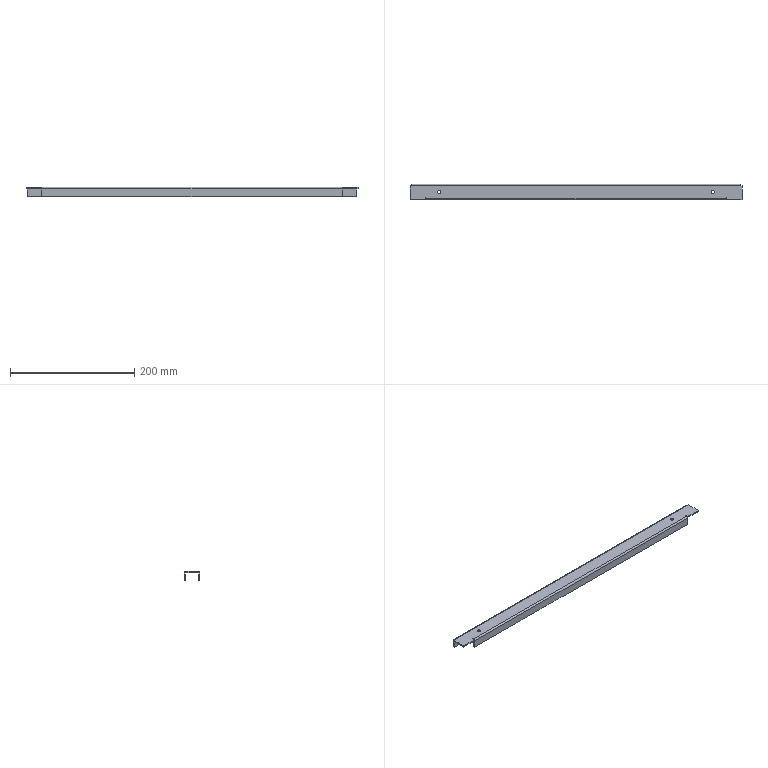Part | STEP file | Clamp Frame Weldment 1 | 1 solid | 30 faces | box 534 x 25 x 15 mm | volume 51628 mm3 | plane 20 | cylinder 10 | commonest cylinder face diameters 1 x4 5.2 x4 5 x2
STEP:
#1=CARTESIAN_POINT('',(-67.6,850.6,-2.));
#2=VERTEX_POINT('',#1);
#3=CARTESIAN_POINT('',(-62.4,850.6,-2.));
#4=VERTEX_POINT('',#3);
#5=CARTESIAN_POINT('',(-65.,850.6,-2.));
#6=DIRECTION('',(0.,0.,1.));
#7=DIRECTION('',(1.,0.,0.));
#8=AXIS2_PLACEMENT_3D('',#5,#6,#7);
#9=CIRCLE('',#8,2.6);
#10=EDGE_CURVE('',#2,#4,#9,.T.);
#11=ORIENTED_EDGE('',*,*,#10,.F.);
#12=CARTESIAN_POINT('',(-67.6,850.6,0.));
#13=VERTEX_POINT('',#12);
#14=CARTESIAN_POINT('',(-67.6,850.6,-10.));
#15=DIRECTION('',(0.,0.,1.));
#16=VECTOR('',#15,1000.);
#17=LINE('',#14,#16);
#18=EDGE_CURVE('',#2,#13,#17,.T.);
#19=ORIENTED_EDGE('',*,*,#18,.T.);
#20=CARTESIAN_POINT('',(-62.4,850.6,0.));
#21=VERTEX_POINT('',#20);
#22=CARTESIAN_POINT('',(-65.,850.6,0.));
#23=DIRECTION('',(0.,0.,1.));
#24=DIRECTION('',(1.,0.,0.));
#25=AXIS2_PLACEMENT_3D('',#22,#23,#24);
#26=CIRCLE('',#25,2.6);
#27=EDGE_CURVE('',#13,#21,#26,.T.);
#28=ORIENTED_EDGE('',*,*,#27,.T.);
#29=CARTESIAN_POINT('',(-62.4,850.6,-10.));
#30=DIRECTION('',(0.,0.,1.));
#31=VECTOR('',#30,1000.);
#32=LINE('',#29,#31);
#33=EDGE_CURVE('',#4,#21,#32,.T.);
#34=ORIENTED_EDGE('',*,*,#33,.F.);
#35=EDGE_LOOP('',(#11,#19,#28,#34));
#36=FACE_OUTER_BOUND('',#35,.T.);
#37=CARTESIAN_POINT('',(-65.,850.6,-10.));
#38=DIRECTION('',(0.,0.,1.));
#39=DIRECTION('',(1.,0.,0.));
#40=AXIS2_PLACEMENT_3D('',#37,#38,#39);
#41=CYLINDRICAL_SURFACE('',#40,2.6);
#42=ADVANCED_FACE('',(#36),#41,.F.);
#43=CARTESIAN_POINT('',(-507.6,850.6,-2.));
#44=VERTEX_POINT('',#43);
#45=CARTESIAN_POINT('',(-502.4,850.6,-2.));
#46=VERTEX_POINT('',#45);
#47=CARTESIAN_POINT('',(-505.,850.6,-2.));
#48=DIRECTION('',(0.,0.,1.));
#49=DIRECTION('',(1.,0.,0.));
#50=AXIS2_PLACEMENT_3D('',#47,#48,#49);
#51=CIRCLE('',#50,2.6);
#52=EDGE_CURVE('',#44,#46,#51,.T.);
#53=ORIENTED_EDGE('',*,*,#52,.F.);
#54=CARTESIAN_POINT('',(-507.6,850.6,0.));
#55=VERTEX_POINT('',#54);
#56=CARTESIAN_POINT('',(-507.6,850.6,-10.));
#57=DIRECTION('',(0.,0.,1.));
#58=VECTOR('',#57,1000.);
#59=LINE('',#56,#58);
#60=EDGE_CURVE('',#44,#55,#59,.T.);
#61=ORIENTED_EDGE('',*,*,#60,.T.);
#62=CARTESIAN_POINT('',(-502.4,850.6,0.));
#63=VERTEX_POINT('',#62);
#64=CARTESIAN_POINT('',(-505.,850.6,0.));
#65=DIRECTION('',(0.,0.,1.));
#66=DIRECTION('',(1.,0.,0.));
#67=AXIS2_PLACEMENT_3D('',#64,#65,#66);
#68=CIRCLE('',#67,2.6);
#69=EDGE_CURVE('',#55,#63,#68,.T.);
#70=ORIENTED_EDGE('',*,*,#69,.T.);
#71=CARTESIAN_POINT('',(-502.4,850.6,-10.));
#72=DIRECTION('',(0.,0.,1.));
#73=VECTOR('',#72,1000.);
#74=LINE('',#71,#73);
#75=EDGE_CURVE('',#46,#63,#74,.T.);
#76=ORIENTED_EDGE('',*,*,#75,.F.);
#77=EDGE_LOOP('',(#53,#61,#70,#76));
#78=FACE_OUTER_BOUND('',#77,.T.);
#79=CARTESIAN_POINT('',(-505.,850.6,-10.));
#80=DIRECTION('',(0.,0.,1.));
#81=DIRECTION('',(1.,0.,0.));
#82=AXIS2_PLACEMENT_3D('',#79,#80,#81);
#83=CYLINDRICAL_SURFACE('',#82,2.6);
#84=ADVANCED_FACE('',(#78),#83,.F.);
#85=CARTESIAN_POINT('',(-527.8,841.6,0.));
#86=VERTEX_POINT('',#85);
#87=CARTESIAN_POINT('',(-526.8,841.6,0.));
#88=VERTEX_POINT('',#87);
#89=CARTESIAN_POINT('',(-527.3,841.6,0.));
#90=DIRECTION('',(0.,0.,-1.));
#91=DIRECTION('',(1.,0.,0.));
#92=AXIS2_PLACEMENT_3D('',#89,#90,#91);
#93=CIRCLE('',#92,0.5);
#94=EDGE_CURVE('',#86,#88,#93,.T.);
#95=ORIENTED_EDGE('',*,*,#94,.T.);
#96=CARTESIAN_POINT('',(-526.8,840.6,0.));
#97=VERTEX_POINT('',#96);
#98=CARTESIAN_POINT('',(-526.8,841.6,0.));
#99=DIRECTION('',(0.,1.,0.));
#100=VECTOR('',#99,1000.);
#101=LINE('',#98,#100);
#102=EDGE_CURVE('',#97,#88,#101,.T.);
#103=ORIENTED_EDGE('',*,*,#102,.F.);
#104=CARTESIAN_POINT('',(-43.2,840.6,0.));
#105=VERTEX_POINT('',#104);
#106=CARTESIAN_POINT('',(0.,840.6,0.));
#107=DIRECTION('',(-1.,0.,0.));
#108=VECTOR('',#107,1000.);
#109=LINE('',#106,#108);
#110=EDGE_CURVE('',#105,#97,#109,.T.);
#111=ORIENTED_EDGE('',*,*,#110,.F.);
#112=CARTESIAN_POINT('',(-43.2,841.6,0.));
#113=VERTEX_POINT('',#112);
#114=CARTESIAN_POINT('',(-43.2,840.6,0.));
#115=DIRECTION('',(0.,-1.,0.));
#116=VECTOR('',#115,1000.);
#117=LINE('',#114,#116);
#118=EDGE_CURVE('',#113,#105,#117,.T.);
#119=ORIENTED_EDGE('',*,*,#118,.F.);
#120=CARTESIAN_POINT('',(-42.2,841.6,0.));
#121=VERTEX_POINT('',#120);
#122=CARTESIAN_POINT('',(-42.7,841.6,0.));
#123=DIRECTION('',(0.,0.,-1.));
#124=DIRECTION('',(1.,0.,0.));
#125=AXIS2_PLACEMENT_3D('',#122,#123,#124);
#126=CIRCLE('',#125,0.5);
#127=EDGE_CURVE('',#113,#121,#126,.T.);
#128=ORIENTED_EDGE('',*,*,#127,.T.);
#129=CARTESIAN_POINT('',(-42.2,838.1,0.));
#130=VERTEX_POINT('',#129);
#131=CARTESIAN_POINT('',(-42.2,0.,0.));
#132=DIRECTION('',(0.,1.,0.));
#133=VECTOR('',#132,1000.);
#134=LINE('',#131,#133);
#135=EDGE_CURVE('',#130,#121,#134,.T.);
#136=ORIENTED_EDGE('',*,*,#135,.F.);
#137=CARTESIAN_POINT('',(-18.,838.1,0.));
#138=VERTEX_POINT('',#137);
#139=CARTESIAN_POINT('',(0.,838.1,0.));
#140=DIRECTION('',(-1.,0.,0.));
#141=VECTOR('',#140,1000.);
#142=LINE('',#139,#141);
#143=EDGE_CURVE('',#138,#130,#142,.T.);
#144=ORIENTED_EDGE('',*,*,#143,.F.);
#145=CARTESIAN_POINT('',(-18.,860.6,0.));
#146=VERTEX_POINT('',#145);
#147=CARTESIAN_POINT('',(-18.,0.,0.));
#148=DIRECTION('',(0.,-1.,0.));
#149=VECTOR('',#148,1000.);
#150=LINE('',#147,#149);
#151=EDGE_CURVE('',#146,#138,#150,.T.);
#152=ORIENTED_EDGE('',*,*,#151,.F.);
#153=CARTESIAN_POINT('',(-20.,860.6,0.));
#154=VERTEX_POINT('',#153);
#155=CARTESIAN_POINT('',(0.,860.6,0.));
#156=DIRECTION('',(1.,0.,0.));
#157=VECTOR('',#156,1000.);
#158=LINE('',#155,#157);
#159=EDGE_CURVE('',#154,#146,#158,.T.);
#160=ORIENTED_EDGE('',*,*,#159,.F.);
#161=CARTESIAN_POINT('',(-550.,860.6,0.));
#162=VERTEX_POINT('',#161);
#163=CARTESIAN_POINT('',(0.,860.6,0.));
#164=DIRECTION('',(1.,0.,0.));
#165=VECTOR('',#164,1000.);
#166=LINE('',#163,#165);
#167=EDGE_CURVE('',#162,#154,#166,.T.);
#168=ORIENTED_EDGE('',*,*,#167,.F.);
#169=CARTESIAN_POINT('',(-552.,860.6,0.));
#170=VERTEX_POINT('',#169);
#171=CARTESIAN_POINT('',(0.,860.6,0.));
#172=DIRECTION('',(1.,0.,0.));
#173=VECTOR('',#172,1000.);
#174=LINE('',#171,#173);
#175=EDGE_CURVE('',#170,#162,#174,.T.);
#176=ORIENTED_EDGE('',*,*,#175,.F.);
#177=CARTESIAN_POINT('',(-552.,838.1,0.));
#178=VERTEX_POINT('',#177);
#179=CARTESIAN_POINT('',(-552.,0.,0.));
#180=DIRECTION('',(0.,1.,0.));
#181=VECTOR('',#180,1000.);
#182=LINE('',#179,#181);
#183=EDGE_CURVE('',#178,#170,#182,.T.);
#184=ORIENTED_EDGE('',*,*,#183,.F.);
#185=CARTESIAN_POINT('',(-527.8,838.1,0.));
#186=VERTEX_POINT('',#185);
#187=CARTESIAN_POINT('',(0.,838.1,0.));
#188=DIRECTION('',(-1.,0.,0.));
#189=VECTOR('',#188,1000.);
#190=LINE('',#187,#189);
#191=EDGE_CURVE('',#186,#178,#190,.T.);
#192=ORIENTED_EDGE('',*,*,#191,.F.);
#193=CARTESIAN_POINT('',(-527.8,0.,0.));
#194=DIRECTION('',(0.,-1.,0.));
#195=VECTOR('',#194,1000.);
#196=LINE('',#193,#195);
#197=EDGE_CURVE('',#86,#186,#196,.T.);
#198=ORIENTED_EDGE('',*,*,#197,.F.);
#199=EDGE_LOOP('',(#95,#103,#111,#119,#128,#136,#144,#152,#160,#168,#176,#184,#192,#198));
#200=FACE_OUTER_BOUND('',#199,.T.);
#201=CARTESIAN_POINT('',(-65.,850.6,0.));
#202=DIRECTION('',(0.,0.,1.));
#203=DIRECTION('',(1.,0.,0.));
#204=AXIS2_PLACEMENT_3D('',#201,#202,#203);
#205=CIRCLE('',#204,2.6);
#206=EDGE_CURVE('',#21,#13,#205,.T.);
#207=ORIENTED_EDGE('',*,*,#206,.F.);
#208=ORIENTED_EDGE('',*,*,#27,.F.);
#209=EDGE_LOOP('',(#207,#208));
#210=FACE_BOUND('',#209,.T.);
#211=CARTESIAN_POINT('',(-505.,850.6,0.));
#212=DIRECTION('',(0.,0.,1.));
#213=DIRECTION('',(1.,0.,0.));
#214=AXIS2_PLACEMENT_3D('',#211,#212,#213);
#215=CIRCLE('',#214,2.6);
#216=EDGE_CURVE('',#63,#55,#215,.T.);
#217=ORIENTED_EDGE('',*,*,#216,.F.);
#218=ORIENTED_EDGE('',*,*,#69,.F.);
#219=EDGE_LOOP('',(#217,#218));
#220=FACE_BOUND('',#219,.T.);
#221=CARTESIAN_POINT('',(0.,0.,0.));
#222=DIRECTION('',(0.,0.,-1.));
#223=DIRECTION('',(-1.,0.,0.));
#224=AXIS2_PLACEMENT_3D('',#221,#222,#223);
#225=PLANE('',#224);
#226=ADVANCED_FACE('',(#200,#210,#220),#225,.F.);
#227=CARTESIAN_POINT('',(-527.8,838.1,-2.));
#228=VERTEX_POINT('',#227);
#229=CARTESIAN_POINT('',(-527.8,838.1,-2.));
#230=DIRECTION('',(0.,0.,-1.));
#231=VECTOR('',#230,1000.);
#232=LINE('',#229,#231);
#233=EDGE_CURVE('',#186,#228,#232,.T.);
#234=ORIENTED_EDGE('',*,*,#233,.T.);
#235=CARTESIAN_POINT('',(-527.8,841.6,-2.));
#236=VERTEX_POINT('',#235);
#237=CARTESIAN_POINT('',(-527.8,838.1,-2.));
#238=DIRECTION('',(0.,1.,0.));
#239=VECTOR('',#238,1000.);
#240=LINE('',#237,#239);
#241=EDGE_CURVE('',#228,#236,#240,.T.);
#242=ORIENTED_EDGE('',*,*,#241,.T.);
#243=CARTESIAN_POINT('',(-527.8,841.6,-2.));
#244=DIRECTION('',(0.,0.,1.));
#245=VECTOR('',#244,1000.);
#246=LINE('',#243,#245);
#247=EDGE_CURVE('',#236,#86,#246,.T.);
#248=ORIENTED_EDGE('',*,*,#247,.T.);
#249=ORIENTED_EDGE('',*,*,#197,.T.);
#250=EDGE_LOOP('',(#234,#242,#248,#249));
#251=FACE_OUTER_BOUND('',#250,.T.);
#252=CARTESIAN_POINT('',(-527.8,838.1,-2.));
#253=DIRECTION('',(1.,0.,0.));
#254=DIRECTION('',(0.,0.,-1.));
#255=AXIS2_PLACEMENT_3D('',#252,#253,#254);
#256=PLANE('',#255);
#257=ADVANCED_FACE('',(#251),#256,.T.);
#258=CARTESIAN_POINT('',(-526.8,838.1,-2.5));
#259=VERTEX_POINT('',#258);
#260=CARTESIAN_POINT('',(-43.2,838.1,-2.5));
#261=VERTEX_POINT('',#260);
#262=CARTESIAN_POINT('',(-526.8,838.1,-2.5));
#263=DIRECTION('',(1.,0.,0.));
#264=VECTOR('',#263,1000.);
#265=LINE('',#262,#264);
#266=EDGE_CURVE('',#259,#261,#265,.T.);
#267=ORIENTED_EDGE('',*,*,#266,.T.);
#268=CARTESIAN_POINT('',(-43.2,840.6,-2.5));
#269=DIRECTION('',(-1.,0.,0.));
#270=DIRECTION('',(0.,0.,1.));
#271=AXIS2_PLACEMENT_3D('',#268,#269,#270);
#272=CIRCLE('',#271,2.5);
#273=EDGE_CURVE('',#261,#105,#272,.T.);
#274=ORIENTED_EDGE('',*,*,#273,.T.);
#275=ORIENTED_EDGE('',*,*,#110,.T.);
#276=CARTESIAN_POINT('',(-526.8,840.6,-2.5));
#277=DIRECTION('',(1.,0.,0.));
#278=DIRECTION('',(0.,0.,1.));
#279=AXIS2_PLACEMENT_3D('',#276,#277,#278);
#280=CIRCLE('',#279,2.5);
#281=EDGE_CURVE('',#97,#259,#280,.T.);
#282=ORIENTED_EDGE('',*,*,#281,.T.);
#283=EDGE_LOOP('',(#267,#274,#275,#282));
#284=FACE_OUTER_BOUND('',#283,.T.);
#285=CARTESIAN_POINT('',(-526.8,840.6,-2.5));
#286=DIRECTION('',(-1.,0.,0.));
#287=DIRECTION('',(0.,0.,1.));
#288=AXIS2_PLACEMENT_3D('',#285,#286,#287);
#289=CYLINDRICAL_SURFACE('',#288,2.5);
#290=ADVANCED_FACE('',(#284),#289,.T.);
#291=CARTESIAN_POINT('',(-42.2,841.6,-2.));
#292=VERTEX_POINT('',#291);
#293=CARTESIAN_POINT('',(-42.2,841.6,-2.));
#294=DIRECTION('',(0.,0.,-1.));
#295=VECTOR('',#294,1000.);
#296=LINE('',#293,#295);
#297=EDGE_CURVE('',#121,#292,#296,.T.);
#298=ORIENTED_EDGE('',*,*,#297,.T.);
#299=CARTESIAN_POINT('',(-42.2,838.1,-2.));
#300=VERTEX_POINT('',#299);
#301=CARTESIAN_POINT('',(-42.2,841.6,-2.));
#302=DIRECTION('',(0.,-1.,0.));
#303=VECTOR('',#302,1000.);
#304=LINE('',#301,#303);
#305=EDGE_CURVE('',#292,#300,#304,.T.);
#306=ORIENTED_EDGE('',*,*,#305,.T.);
#307=CARTESIAN_POINT('',(-42.2,838.1,-2.));
#308=DIRECTION('',(0.,0.,1.));
#309=VECTOR('',#308,1000.);
#310=LINE('',#307,#309);
#311=EDGE_CURVE('',#300,#130,#310,.T.);
#312=ORIENTED_EDGE('',*,*,#311,.T.);
#313=ORIENTED_EDGE('',*,*,#135,.T.);
#314=EDGE_LOOP('',(#298,#306,#312,#313));
#315=FACE_OUTER_BOUND('',#314,.T.);
#316=CARTESIAN_POINT('',(-42.2,841.6,-2.));
#317=DIRECTION('',(-1.,0.,0.));
#318=DIRECTION('',(0.,0.,1.));
#319=AXIS2_PLACEMENT_3D('',#316,#317,#318);
#320=PLANE('',#319);
#321=ADVANCED_FACE('',(#315),#320,.T.);
#322=CARTESIAN_POINT('',(-18.,838.1,-2.));
#323=VERTEX_POINT('',#322);
#324=CARTESIAN_POINT('',(-18.,838.1,-2.));
#325=DIRECTION('',(0.,0.,1.));
#326=VECTOR('',#325,1000.);
#327=LINE('',#324,#326);
#328=EDGE_CURVE('',#323,#138,#327,.T.);
#329=ORIENTED_EDGE('',*,*,#328,.T.);
#330=ORIENTED_EDGE('',*,*,#143,.T.);
#331=ORIENTED_EDGE('',*,*,#311,.F.);
#332=CARTESIAN_POINT('',(-43.,838.1,-2.));
#333=DIRECTION('',(1.,0.,0.));
#334=VECTOR('',#333,1000.);
#335=LINE('',#332,#334);
#336=EDGE_CURVE('',#300,#323,#335,.T.);
#337=ORIENTED_EDGE('',*,*,#336,.T.);
#338=EDGE_LOOP('',(#329,#330,#331,#337));
#339=FACE_OUTER_BOUND('',#338,.T.);
#340=CARTESIAN_POINT('',(-43.,838.1,-2.));
#341=DIRECTION('',(0.,-1.,0.));
#342=DIRECTION('',(0.,0.,-1.));
#343=AXIS2_PLACEMENT_3D('',#340,#341,#342);
#344=PLANE('',#343);
#345=ADVANCED_FACE('',(#339),#344,.T.);
#346=CARTESIAN_POINT('',(-18.,860.6,-2.));
#347=VERTEX_POINT('',#346);
#348=CARTESIAN_POINT('',(-18.,860.6,0.));
#349=DIRECTION('',(0.,0.,1.));
#350=VECTOR('',#349,1000.);
#351=LINE('',#348,#350);
#352=EDGE_CURVE('',#347,#146,#351,.T.);
#353=ORIENTED_EDGE('',*,*,#352,.T.);
#354=ORIENTED_EDGE('',*,*,#151,.T.);
#355=ORIENTED_EDGE('',*,*,#328,.F.);
#356=CARTESIAN_POINT('',(-18.,0.,-2.));
#357=DIRECTION('',(0.,1.,0.));
#358=VECTOR('',#357,1000.);
#359=LINE('',#356,#358);
#360=EDGE_CURVE('',#323,#347,#359,.T.);
#361=ORIENTED_EDGE('',*,*,#360,.T.);
#362=EDGE_LOOP('',(#353,#354,#355,#361));
#363=FACE_OUTER_BOUND('',#362,.T.);
#364=CARTESIAN_POINT('',(-18.,0.,0.));
#365=DIRECTION('',(1.,0.,0.));
#366=DIRECTION('',(0.,1.,0.));
#367=AXIS2_PLACEMENT_3D('',#364,#365,#366);
#368=PLANE('',#367);
#369=ADVANCED_FACE('',(#363),#368,.T.);
#370=ORIENTED_EDGE('',*,*,#159,.T.);
#371=ORIENTED_EDGE('',*,*,#352,.F.);
#372=CARTESIAN_POINT('',(-20.,860.6,-2.));
#373=VERTEX_POINT('',#372);
#374=CARTESIAN_POINT('',(-18.,860.6,-2.));
#375=DIRECTION('',(1.,0.,0.));
#376=VECTOR('',#375,1000.);
#377=LINE('',#374,#376);
#378=EDGE_CURVE('',#373,#347,#377,.T.);
#379=ORIENTED_EDGE('',*,*,#378,.F.);
#380=CARTESIAN_POINT('',(-20.,860.6,-2.));
#381=DIRECTION('',(0.,0.,-1.));
#382=VECTOR('',#381,1000.);
#383=LINE('',#380,#382);
#384=EDGE_CURVE('',#154,#373,#383,.T.);
#385=ORIENTED_EDGE('',*,*,#384,.F.);
#386=EDGE_LOOP('',(#370,#371,#379,#385));
#387=FACE_OUTER_BOUND('',#386,.T.);
#388=CARTESIAN_POINT('',(-18.,860.6,-2.));
#389=DIRECTION('',(0.,-1.,0.));
#390=DIRECTION('',(1.,0.,0.));
#391=AXIS2_PLACEMENT_3D('',#388,#389,#390);
#392=PLANE('',#391);
#393=ADVANCED_FACE('',(#387),#392,.F.);
#394=CARTESIAN_POINT('',(-20.,863.1,-2.5));
#395=VERTEX_POINT('',#394);
#396=CARTESIAN_POINT('',(-550.,863.1,-2.5));
#397=VERTEX_POINT('',#396);
#398=CARTESIAN_POINT('',(-20.,863.1,-2.5));
#399=DIRECTION('',(-1.,0.,0.));
#400=VECTOR('',#399,1000.);
#401=LINE('',#398,#400);
#402=EDGE_CURVE('',#395,#397,#401,.T.);
#403=ORIENTED_EDGE('',*,*,#402,.T.);
#404=CARTESIAN_POINT('',(-550.,860.6,-2.5));
#405=DIRECTION('',(1.,0.,0.));
#406=DIRECTION('',(0.,0.,-1.));
#407=AXIS2_PLACEMENT_3D('',#404,#405,#406);
#408=CIRCLE('',#407,2.5);
#409=EDGE_CURVE('',#397,#162,#408,.T.);
#410=ORIENTED_EDGE('',*,*,#409,.T.);
#411=ORIENTED_EDGE('',*,*,#167,.T.);
#412=CARTESIAN_POINT('',(-20.,860.6,-2.5));
#413=DIRECTION('',(-1.,0.,0.));
#414=DIRECTION('',(0.,0.,-1.));
#415=AXIS2_PLACEMENT_3D('',#412,#413,#414);
#416=CIRCLE('',#415,2.5);
#417=EDGE_CURVE('',#154,#395,#416,.T.);
#418=ORIENTED_EDGE('',*,*,#417,.T.);
#419=EDGE_LOOP('',(#403,#410,#411,#418));
#420=FACE_OUTER_BOUND('',#419,.T.);
#421=CARTESIAN_POINT('',(-20.,860.6,-2.5));
#422=DIRECTION('',(1.,0.,0.));
#423=DIRECTION('',(0.,0.,-1.));
#424=AXIS2_PLACEMENT_3D('',#421,#422,#423);
#425=CYLINDRICAL_SURFACE('',#424,2.5);
#426=ADVANCED_FACE('',(#420),#425,.T.);
#427=CARTESIAN_POINT('',(-552.,860.6,-2.));
#428=VERTEX_POINT('',#427);
#429=CARTESIAN_POINT('',(-550.,860.6,-2.));
#430=VERTEX_POINT('',#429);
#431=CARTESIAN_POINT('',(-552.,860.6,-2.));
#432=DIRECTION('',(1.,0.,0.));
#433=VECTOR('',#432,1000.);
#434=LINE('',#431,#433);
#435=EDGE_CURVE('',#428,#430,#434,.T.);
#436=ORIENTED_EDGE('',*,*,#435,.F.);
#437=CARTESIAN_POINT('',(-552.,860.6,0.));
#438=DIRECTION('',(0.,0.,-1.));
#439=VECTOR('',#438,1000.);
#440=LINE('',#437,#439);
#441=EDGE_CURVE('',#170,#428,#440,.T.);
#442=ORIENTED_EDGE('',*,*,#441,.F.);
#443=ORIENTED_EDGE('',*,*,#175,.T.);
#444=CARTESIAN_POINT('',(-550.,860.6,0.));
#445=DIRECTION('',(0.,0.,1.));
#446=VECTOR('',#445,1000.);
#447=LINE('',#444,#446);
#448=EDGE_CURVE('',#430,#162,#447,.T.);
#449=ORIENTED_EDGE('',*,*,#448,.F.);
#450=EDGE_LOOP('',(#436,#442,#443,#449));
#451=FACE_OUTER_BOUND('',#450,.T.);
#452=CARTESIAN_POINT('',(-552.,860.6,0.));
#453=DIRECTION('',(0.,-1.,0.));
#454=DIRECTION('',(0.,0.,-1.));
#455=AXIS2_PLACEMENT_3D('',#452,#453,#454);
#456=PLANE('',#455);
#457=ADVANCED_FACE('',(#451),#456,.F.);
#458=CARTESIAN_POINT('',(-552.,838.1,-2.));
#459=VERTEX_POINT('',#458);
#460=CARTESIAN_POINT('',(-552.,0.,-2.));
#461=DIRECTION('',(0.,-1.,0.));
#462=VECTOR('',#461,1000.);
#463=LINE('',#460,#462);
#464=EDGE_CURVE('',#428,#459,#463,.T.);
#465=ORIENTED_EDGE('',*,*,#464,.T.);
#466=CARTESIAN_POINT('',(-552.,838.1,0.));
#467=DIRECTION('',(0.,0.,1.));
#468=VECTOR('',#467,1000.);
#469=LINE('',#466,#468);
#470=EDGE_CURVE('',#459,#178,#469,.T.);
#471=ORIENTED_EDGE('',*,*,#470,.T.);
#472=ORIENTED_EDGE('',*,*,#183,.T.);
#473=ORIENTED_EDGE('',*,*,#441,.T.);
#474=EDGE_LOOP('',(#465,#471,#472,#473));
#475=FACE_OUTER_BOUND('',#474,.T.);
#476=CARTESIAN_POINT('',(-552.,0.,0.));
#477=DIRECTION('',(-1.,0.,0.));
#478=DIRECTION('',(0.,0.,1.));
#479=AXIS2_PLACEMENT_3D('',#476,#477,#478);
#480=PLANE('',#479);
#481=ADVANCED_FACE('',(#475),#480,.T.);
#482=ORIENTED_EDGE('',*,*,#191,.T.);
#483=ORIENTED_EDGE('',*,*,#470,.F.);
#484=CARTESIAN_POINT('',(-550.,838.1,-2.));
#485=DIRECTION('',(1.,0.,0.));
#486=VECTOR('',#485,1000.);
#487=LINE('',#484,#486);
#488=EDGE_CURVE('',#459,#228,#487,.T.);
#489=ORIENTED_EDGE('',*,*,#488,.T.);
#490=ORIENTED_EDGE('',*,*,#233,.F.);
#491=EDGE_LOOP('',(#482,#483,#489,#490));
#492=FACE_OUTER_BOUND('',#491,.T.);
#493=CARTESIAN_POINT('',(-550.,838.1,-2.));
#494=DIRECTION('',(0.,-1.,0.));
#495=DIRECTION('',(1.,0.,0.));
#496=AXIS2_PLACEMENT_3D('',#493,#494,#495);
#497=PLANE('',#496);
#498=ADVANCED_FACE('',(#492),#497,.T.);
#499=ORIENTED_EDGE('',*,*,#18,.F.);
#500=CARTESIAN_POINT('',(-65.,850.6,-2.));
#501=DIRECTION('',(0.,0.,1.));
#502=DIRECTION('',(1.,0.,0.));
#503=AXIS2_PLACEMENT_3D('',#500,#501,#502);
#504=CIRCLE('',#503,2.6);
#505=EDGE_CURVE('',#4,#2,#504,.T.);
#506=ORIENTED_EDGE('',*,*,#505,.F.);
#507=ORIENTED_EDGE('',*,*,#33,.T.);
#508=ORIENTED_EDGE('',*,*,#206,.T.);
#509=EDGE_LOOP('',(#499,#506,#507,#508));
#510=FACE_OUTER_BOUND('',#509,.T.);
#511=CARTESIAN_POINT('',(-65.,850.6,-10.));
#512=DIRECTION('',(0.,0.,1.));
#513=DIRECTION('',(1.,0.,0.));
#514=AXIS2_PLACEMENT_3D('',#511,#512,#513);
#515=CYLINDRICAL_SURFACE('',#514,2.6);
#516=ADVANCED_FACE('',(#510),#515,.F.);
#517=ORIENTED_EDGE('',*,*,#60,.F.);
#518=CARTESIAN_POINT('',(-505.,850.6,-2.));
#519=DIRECTION('',(0.,0.,1.));
#520=DIRECTION('',(1.,0.,0.));
#521=AXIS2_PLACEMENT_3D('',#518,#519,#520);
#522=CIRCLE('',#521,2.6);
#523=EDGE_CURVE('',#46,#44,#522,.T.);
#524=ORIENTED_EDGE('',*,*,#523,.F.);
#525=ORIENTED_EDGE('',*,*,#75,.T.);
#526=ORIENTED_EDGE('',*,*,#216,.T.);
#527=EDGE_LOOP('',(#517,#524,#525,#526));
#528=FACE_OUTER_BOUND('',#527,.T.);
#529=CARTESIAN_POINT('',(-505.,850.6,-10.));
#530=DIRECTION('',(0.,0.,1.));
#531=DIRECTION('',(1.,0.,0.));
#532=AXIS2_PLACEMENT_3D('',#529,#530,#531);
#533=CYLINDRICAL_SURFACE('',#532,2.6);
#534=ADVANCED_FACE('',(#528),#533,.F.);
#535=CARTESIAN_POINT('',(-43.2,840.6,-2.));
#536=VERTEX_POINT('',#535);
#537=CARTESIAN_POINT('',(-526.8,840.6,-2.));
#538=VERTEX_POINT('',#537);
#539=CARTESIAN_POINT('',(0.,840.6,-2.));
#540=DIRECTION('',(-1.,0.,0.));
#541=VECTOR('',#540,1000.);
#542=LINE('',#539,#541);
#543=EDGE_CURVE('',#536,#538,#542,.T.);
#544=ORIENTED_EDGE('',*,*,#543,.T.);
#545=CARTESIAN_POINT('',(-526.8,841.6,-2.));
#546=VERTEX_POINT('',#545);
#547=CARTESIAN_POINT('',(-526.8,841.6,-2.));
#548=DIRECTION('',(0.,-1.,0.));
#549=VECTOR('',#548,1000.);
#550=LINE('',#547,#549);
#551=EDGE_CURVE('',#546,#538,#550,.T.);
#552=ORIENTED_EDGE('',*,*,#551,.F.);
#553=CARTESIAN_POINT('',(-527.3,841.6,-2.));
#554=DIRECTION('',(0.,0.,1.));
#555=DIRECTION('',(1.,0.,0.));
#556=AXIS2_PLACEMENT_3D('',#553,#554,#555);
#557=CIRCLE('',#556,0.5);
#558=EDGE_CURVE('',#546,#236,#557,.T.);
#559=ORIENTED_EDGE('',*,*,#558,.T.);
#560=ORIENTED_EDGE('',*,*,#241,.F.);
#561=ORIENTED_EDGE('',*,*,#488,.F.);
#562=ORIENTED_EDGE('',*,*,#464,.F.);
#563=ORIENTED_EDGE('',*,*,#435,.T.);
#564=CARTESIAN_POINT('',(0.,860.6,-2.));
#565=DIRECTION('',(1.,0.,0.));
#566=VECTOR('',#565,1000.);
#567=LINE('',#564,#566);
#568=EDGE_CURVE('',#430,#373,#567,.T.);
#569=ORIENTED_EDGE('',*,*,#568,.T.);
#570=ORIENTED_EDGE('',*,*,#378,.T.);
#571=ORIENTED_EDGE('',*,*,#360,.F.);
#572=ORIENTED_EDGE('',*,*,#336,.F.);
#573=ORIENTED_EDGE('',*,*,#305,.F.);
#574=CARTESIAN_POINT('',(-43.2,841.6,-2.));
#575=VERTEX_POINT('',#574);
#576=CARTESIAN_POINT('',(-42.7,841.6,-2.));
#577=DIRECTION('',(0.,0.,1.));
#578=DIRECTION('',(1.,0.,0.));
#579=AXIS2_PLACEMENT_3D('',#576,#577,#578);
#580=CIRCLE('',#579,0.5);
#581=EDGE_CURVE('',#292,#575,#580,.T.);
#582=ORIENTED_EDGE('',*,*,#581,.T.);
#583=CARTESIAN_POINT('',(-43.2,840.6,-2.));
#584=DIRECTION('',(0.,1.,0.));
#585=VECTOR('',#584,1000.);
#586=LINE('',#583,#585);
#587=EDGE_CURVE('',#536,#575,#586,.T.);
#588=ORIENTED_EDGE('',*,*,#587,.F.);
#589=EDGE_LOOP('',(#544,#552,#559,#560,#561,#562,#563,#569,#570,#571,#572,#573,#582,#588));
#590=FACE_OUTER_BOUND('',#589,.T.);
#591=ORIENTED_EDGE('',*,*,#505,.T.);
#592=ORIENTED_EDGE('',*,*,#10,.T.);
#593=EDGE_LOOP('',(#591,#592));
#594=FACE_BOUND('',#593,.T.);
#595=ORIENTED_EDGE('',*,*,#523,.T.);
#596=ORIENTED_EDGE('',*,*,#52,.T.);
#597=EDGE_LOOP('',(#595,#596));
#598=FACE_BOUND('',#597,.T.);
#599=CARTESIAN_POINT('',(0.,0.,-2.));
#600=DIRECTION('',(0.,0.,-1.));
#601=DIRECTION('',(-1.,0.,0.));
#602=AXIS2_PLACEMENT_3D('',#599,#600,#601);
#603=PLANE('',#602);
#604=ADVANCED_FACE('',(#590,#594,#598),#603,.T.);
#605=ORIENTED_EDGE('',*,*,#94,.F.);
#606=ORIENTED_EDGE('',*,*,#247,.F.);
#607=ORIENTED_EDGE('',*,*,#558,.F.);
#608=CARTESIAN_POINT('',(-526.8,841.6,-2.));
#609=DIRECTION('',(0.,0.,-1.));
#610=VECTOR('',#609,1000.);
#611=LINE('',#608,#610);
#612=EDGE_CURVE('',#88,#546,#611,.T.);
#613=ORIENTED_EDGE('',*,*,#612,.F.);
#614=EDGE_LOOP('',(#605,#606,#607,#613));
#615=FACE_OUTER_BOUND('',#614,.T.);
#616=CARTESIAN_POINT('',(-527.3,841.6,-2.));
#617=DIRECTION('',(0.,0.,1.));
#618=DIRECTION('',(1.,0.,0.));
#619=AXIS2_PLACEMENT_3D('',#616,#617,#618);
#620=CYLINDRICAL_SURFACE('',#619,0.5);
#621=ADVANCED_FACE('',(#615),#620,.F.);
#622=CARTESIAN_POINT('',(-43.2,840.1,-2.5));
#623=VERTEX_POINT('',#622);
#624=CARTESIAN_POINT('',(-43.2,840.6,-2.5));
#625=DIRECTION('',(-1.,0.,0.));
#626=DIRECTION('',(0.,0.,1.));
#627=AXIS2_PLACEMENT_3D('',#624,#625,#626);
#628=CIRCLE('',#627,0.5);
#629=EDGE_CURVE('',#623,#536,#628,.T.);
#630=ORIENTED_EDGE('',*,*,#629,.T.);
#631=ORIENTED_EDGE('',*,*,#587,.T.);
#632=CARTESIAN_POINT('',(-43.2,841.6,-2.));
#633=DIRECTION('',(0.,0.,1.));
#634=VECTOR('',#633,1000.);
#635=LINE('',#632,#634);
#636=EDGE_CURVE('',#575,#113,#635,.T.);
#637=ORIENTED_EDGE('',*,*,#636,.T.);
#638=ORIENTED_EDGE('',*,*,#118,.T.);
#639=ORIENTED_EDGE('',*,*,#273,.F.);
#640=CARTESIAN_POINT('',(-43.2,838.1,-15.));
#641=VERTEX_POINT('',#640);
#642=CARTESIAN_POINT('',(-43.2,838.1,0.));
#643=DIRECTION('',(0.,0.,1.));
#644=VECTOR('',#643,1000.);
#645=LINE('',#642,#644);
#646=EDGE_CURVE('',#641,#261,#645,.T.);
#647=ORIENTED_EDGE('',*,*,#646,.F.);
#648=CARTESIAN_POINT('',(-43.2,840.1,-15.));
#649=VERTEX_POINT('',#648);
#650=CARTESIAN_POINT('',(-43.2,838.1,-15.));
#651=DIRECTION('',(0.,1.,0.));
#652=VECTOR('',#651,1000.);
#653=LINE('',#650,#652);
#654=EDGE_CURVE('',#641,#649,#653,.T.);
#655=ORIENTED_EDGE('',*,*,#654,.T.);
#656=CARTESIAN_POINT('',(-43.2,840.1,-15.));
#657=DIRECTION('',(0.,0.,1.));
#658=VECTOR('',#657,1000.);
#659=LINE('',#656,#658);
#660=EDGE_CURVE('',#649,#623,#659,.T.);
#661=ORIENTED_EDGE('',*,*,#660,.T.);
#662=EDGE_LOOP('',(#630,#631,#637,#638,#639,#647,#655,#661));
#663=FACE_OUTER_BOUND('',#662,.T.);
#664=CARTESIAN_POINT('',(-43.2,840.6,-2.5));
#665=DIRECTION('',(1.,0.,0.));
#666=DIRECTION('',(0.,0.,-1.));
#667=AXIS2_PLACEMENT_3D('',#664,#665,#666);
#668=PLANE('',#667);
#669=ADVANCED_FACE('',(#663),#668,.T.);
#670=CARTESIAN_POINT('',(-526.8,838.1,-15.));
#671=VERTEX_POINT('',#670);
#672=CARTESIAN_POINT('',(-526.8,838.1,0.));
#673=DIRECTION('',(0.,0.,-1.));
#674=VECTOR('',#673,1000.);
#675=LINE('',#672,#674);
#676=EDGE_CURVE('',#259,#671,#675,.T.);
#677=ORIENTED_EDGE('',*,*,#676,.T.);
#678=CARTESIAN_POINT('',(0.,838.1,-15.));
#679=DIRECTION('',(1.,0.,0.));
#680=VECTOR('',#679,1000.);
#681=LINE('',#678,#680);
#682=EDGE_CURVE('',#671,#641,#681,.T.);
#683=ORIENTED_EDGE('',*,*,#682,.T.);
#684=ORIENTED_EDGE('',*,*,#646,.T.);
#685=ORIENTED_EDGE('',*,*,#266,.F.);
#686=EDGE_LOOP('',(#677,#683,#684,#685));
#687=FACE_OUTER_BOUND('',#686,.T.);
#688=CARTESIAN_POINT('',(0.,838.1,0.));
#689=DIRECTION('',(0.,-1.,0.));
#690=DIRECTION('',(0.,0.,-1.));
#691=AXIS2_PLACEMENT_3D('',#688,#689,#690);
#692=PLANE('',#691);
#693=ADVANCED_FACE('',(#687),#692,.T.);
#694=CARTESIAN_POINT('',(-526.8,840.1,-2.5));
#695=VERTEX_POINT('',#694);
#696=CARTESIAN_POINT('',(-526.8,840.6,-2.5));
#697=DIRECTION('',(-1.,0.,0.));
#698=DIRECTION('',(0.,0.,1.));
#699=AXIS2_PLACEMENT_3D('',#696,#697,#698);
#700=CIRCLE('',#699,0.5);
#701=EDGE_CURVE('',#695,#538,#700,.T.);
#702=ORIENTED_EDGE('',*,*,#701,.F.);
#703=CARTESIAN_POINT('',(-526.8,840.1,-15.));
#704=VERTEX_POINT('',#703);
#705=CARTESIAN_POINT('',(-526.8,840.1,-2.));
#706=DIRECTION('',(0.,0.,-1.));
#707=VECTOR('',#706,1000.);
#708=LINE('',#705,#707);
#709=EDGE_CURVE('',#695,#704,#708,.T.);
#710=ORIENTED_EDGE('',*,*,#709,.T.);
#711=CARTESIAN_POINT('',(-526.8,838.1,-15.));
#712=DIRECTION('',(0.,1.,0.));
#713=VECTOR('',#712,1000.);
#714=LINE('',#711,#713);
#715=EDGE_CURVE('',#671,#704,#714,.T.);
#716=ORIENTED_EDGE('',*,*,#715,.F.);
#717=ORIENTED_EDGE('',*,*,#676,.F.);
#718=ORIENTED_EDGE('',*,*,#281,.F.);
#719=ORIENTED_EDGE('',*,*,#102,.T.);
#720=ORIENTED_EDGE('',*,*,#612,.T.);
#721=ORIENTED_EDGE('',*,*,#551,.T.);
#722=EDGE_LOOP('',(#702,#710,#716,#717,#718,#719,#720,#721));
#723=FACE_OUTER_BOUND('',#722,.T.);
#724=CARTESIAN_POINT('',(-526.8,840.6,-2.5));
#725=DIRECTION('',(1.,0.,0.));
#726=DIRECTION('',(0.,0.,-1.));
#727=AXIS2_PLACEMENT_3D('',#724,#725,#726);
#728=PLANE('',#727);
#729=ADVANCED_FACE('',(#723),#728,.F.);
#730=ORIENTED_EDGE('',*,*,#127,.F.);
#731=ORIENTED_EDGE('',*,*,#636,.F.);
#732=ORIENTED_EDGE('',*,*,#581,.F.);
#733=ORIENTED_EDGE('',*,*,#297,.F.);
#734=EDGE_LOOP('',(#730,#731,#732,#733));
#735=FACE_OUTER_BOUND('',#734,.T.);
#736=CARTESIAN_POINT('',(-42.7,841.6,-2.));
#737=DIRECTION('',(0.,0.,1.));
#738=DIRECTION('',(1.,0.,0.));
#739=AXIS2_PLACEMENT_3D('',#736,#737,#738);
#740=CYLINDRICAL_SURFACE('',#739,0.5);
#741=ADVANCED_FACE('',(#735),#740,.F.);
#742=CARTESIAN_POINT('',(-20.,861.1,-2.5));
#743=VERTEX_POINT('',#742);
#744=CARTESIAN_POINT('',(-20.,860.6,-2.5));
#745=DIRECTION('',(1.,0.,0.));
#746=DIRECTION('',(0.,0.,-1.));
#747=AXIS2_PLACEMENT_3D('',#744,#745,#746);
#748=CIRCLE('',#747,0.5);
#749=EDGE_CURVE('',#743,#373,#748,.T.);
#750=ORIENTED_EDGE('',*,*,#749,.F.);
#751=CARTESIAN_POINT('',(-20.,861.1,-15.));
#752=VERTEX_POINT('',#751);
#753=CARTESIAN_POINT('',(-20.,861.1,-2.));
#754=DIRECTION('',(0.,0.,-1.));
#755=VECTOR('',#754,1000.);
#756=LINE('',#753,#755);
#757=EDGE_CURVE('',#743,#752,#756,.T.);
#758=ORIENTED_EDGE('',*,*,#757,.T.);
#759=CARTESIAN_POINT('',(-20.,863.1,-15.));
#760=VERTEX_POINT('',#759);
#761=CARTESIAN_POINT('',(-20.,863.1,-15.));
#762=DIRECTION('',(0.,1.,0.));
#763=VECTOR('',#762,1000.);
#764=LINE('',#761,#763);
#765=EDGE_CURVE('',#752,#760,#764,.T.);
#766=ORIENTED_EDGE('',*,*,#765,.T.);
#767=CARTESIAN_POINT('',(-20.,863.1,0.));
#768=DIRECTION('',(0.,0.,-1.));
#769=VECTOR('',#768,1000.);
#770=LINE('',#767,#769);
#771=EDGE_CURVE('',#395,#760,#770,.T.);
#772=ORIENTED_EDGE('',*,*,#771,.F.);
#773=ORIENTED_EDGE('',*,*,#417,.F.);
#774=ORIENTED_EDGE('',*,*,#384,.T.);
#775=EDGE_LOOP('',(#750,#758,#766,#772,#773,#774));
#776=FACE_OUTER_BOUND('',#775,.T.);
#777=CARTESIAN_POINT('',(-20.,860.6,-2.5));
#778=DIRECTION('',(-1.,0.,0.));
#779=DIRECTION('',(0.,0.,1.));
#780=AXIS2_PLACEMENT_3D('',#777,#778,#779);
#781=PLANE('',#780);
#782=ADVANCED_FACE('',(#776),#781,.F.);
#783=ORIENTED_EDGE('',*,*,#448,.T.);
#784=ORIENTED_EDGE('',*,*,#409,.F.);
#785=CARTESIAN_POINT('',(-550.,863.1,-15.));
#786=VERTEX_POINT('',#785);
#787=CARTESIAN_POINT('',(-550.,863.1,0.));
#788=DIRECTION('',(0.,0.,1.));
#789=VECTOR('',#788,1000.);
#790=LINE('',#787,#789);
#791=EDGE_CURVE('',#786,#397,#790,.T.);
#792=ORIENTED_EDGE('',*,*,#791,.F.);
#793=CARTESIAN_POINT('',(-550.,861.1,-15.));
#794=VERTEX_POINT('',#793);
#795=CARTESIAN_POINT('',(-550.,863.1,-15.));
#796=DIRECTION('',(0.,-1.,0.));
#797=VECTOR('',#796,1000.);
#798=LINE('',#795,#797);
#799=EDGE_CURVE('',#786,#794,#798,.T.);
#800=ORIENTED_EDGE('',*,*,#799,.T.);
#801=CARTESIAN_POINT('',(-550.,861.1,-2.5));
#802=VERTEX_POINT('',#801);
#803=CARTESIAN_POINT('',(-550.,861.1,-15.));
#804=DIRECTION('',(0.,0.,1.));
#805=VECTOR('',#804,1000.);
#806=LINE('',#803,#805);
#807=EDGE_CURVE('',#794,#802,#806,.T.);
#808=ORIENTED_EDGE('',*,*,#807,.T.);
#809=CARTESIAN_POINT('',(-550.,860.6,-2.5));
#810=DIRECTION('',(1.,0.,0.));
#811=DIRECTION('',(0.,0.,-1.));
#812=AXIS2_PLACEMENT_3D('',#809,#810,#811);
#813=CIRCLE('',#812,0.5);
#814=EDGE_CURVE('',#802,#430,#813,.T.);
#815=ORIENTED_EDGE('',*,*,#814,.T.);
#816=EDGE_LOOP('',(#783,#784,#792,#800,#808,#815));
#817=FACE_OUTER_BOUND('',#816,.T.);
#818=CARTESIAN_POINT('',(-550.,860.6,-2.5));
#819=DIRECTION('',(-1.,0.,0.));
#820=DIRECTION('',(0.,0.,1.));
#821=AXIS2_PLACEMENT_3D('',#818,#819,#820);
#822=PLANE('',#821);
#823=ADVANCED_FACE('',(#817),#822,.T.);
#824=ORIENTED_EDGE('',*,*,#771,.T.);
#825=CARTESIAN_POINT('',(0.,863.1,-15.));
#826=DIRECTION('',(-1.,0.,0.));
#827=VECTOR('',#826,1000.);
#828=LINE('',#825,#827);
#829=EDGE_CURVE('',#760,#786,#828,.T.);
#830=ORIENTED_EDGE('',*,*,#829,.T.);
#831=ORIENTED_EDGE('',*,*,#791,.T.);
#832=ORIENTED_EDGE('',*,*,#402,.F.);
#833=EDGE_LOOP('',(#824,#830,#831,#832));
#834=FACE_OUTER_BOUND('',#833,.T.);
#835=CARTESIAN_POINT('',(0.,863.1,0.));
#836=DIRECTION('',(0.,1.,0.));
#837=DIRECTION('',(0.,0.,1.));
#838=AXIS2_PLACEMENT_3D('',#835,#836,#837);
#839=PLANE('',#838);
#840=ADVANCED_FACE('',(#834),#839,.T.);
#841=ORIENTED_EDGE('',*,*,#629,.F.);
#842=CARTESIAN_POINT('',(-526.8,840.1,-2.5));
#843=DIRECTION('',(1.,0.,0.));
#844=VECTOR('',#843,1000.);
#845=LINE('',#842,#844);
#846=EDGE_CURVE('',#695,#623,#845,.T.);
#847=ORIENTED_EDGE('',*,*,#846,.F.);
#848=ORIENTED_EDGE('',*,*,#701,.T.);
#849=ORIENTED_EDGE('',*,*,#543,.F.);
#850=EDGE_LOOP('',(#841,#847,#848,#849));
#851=FACE_OUTER_BOUND('',#850,.T.);
#852=CARTESIAN_POINT('',(-526.8,840.6,-2.5));
#853=DIRECTION('',(-1.,0.,0.));
#854=DIRECTION('',(0.,0.,1.));
#855=AXIS2_PLACEMENT_3D('',#852,#853,#854);
#856=CYLINDRICAL_SURFACE('',#855,0.5);
#857=ADVANCED_FACE('',(#851),#856,.F.);
#858=ORIENTED_EDGE('',*,*,#814,.F.);
#859=CARTESIAN_POINT('',(-20.,861.1,-2.5));
#860=DIRECTION('',(-1.,0.,0.));
#861=VECTOR('',#860,1000.);
#862=LINE('',#859,#861);
#863=EDGE_CURVE('',#743,#802,#862,.T.);
#864=ORIENTED_EDGE('',*,*,#863,.F.);
#865=ORIENTED_EDGE('',*,*,#749,.T.);
#866=ORIENTED_EDGE('',*,*,#568,.F.);
#867=EDGE_LOOP('',(#858,#864,#865,#866));
#868=FACE_OUTER_BOUND('',#867,.T.);
#869=CARTESIAN_POINT('',(-20.,860.6,-2.5));
#870=DIRECTION('',(1.,0.,0.));
#871=DIRECTION('',(0.,0.,-1.));
#872=AXIS2_PLACEMENT_3D('',#869,#870,#871);
#873=CYLINDRICAL_SURFACE('',#872,0.5);
#874=ADVANCED_FACE('',(#868),#873,.F.);
#875=ORIENTED_EDGE('',*,*,#682,.F.);
#876=ORIENTED_EDGE('',*,*,#715,.T.);
#877=CARTESIAN_POINT('',(-526.8,840.1,-15.));
#878=DIRECTION('',(1.,0.,0.));
#879=VECTOR('',#878,1000.);
#880=LINE('',#877,#879);
#881=EDGE_CURVE('',#704,#649,#880,.T.);
#882=ORIENTED_EDGE('',*,*,#881,.T.);
#883=ORIENTED_EDGE('',*,*,#654,.F.);
#884=EDGE_LOOP('',(#875,#876,#882,#883));
#885=FACE_OUTER_BOUND('',#884,.T.);
#886=CARTESIAN_POINT('',(-526.8,838.1,-15.));
#887=DIRECTION('',(0.,0.,-1.));
#888=DIRECTION('',(0.,1.,0.));
#889=AXIS2_PLACEMENT_3D('',#886,#887,#888);
#890=PLANE('',#889);
#891=ADVANCED_FACE('',(#885),#890,.T.);
#892=ORIENTED_EDGE('',*,*,#829,.F.);
#893=ORIENTED_EDGE('',*,*,#765,.F.);
#894=CARTESIAN_POINT('',(-20.,861.1,-15.));
#895=DIRECTION('',(-1.,0.,0.));
#896=VECTOR('',#895,1000.);
#897=LINE('',#894,#896);
#898=EDGE_CURVE('',#752,#794,#897,.T.);
#899=ORIENTED_EDGE('',*,*,#898,.T.);
#900=ORIENTED_EDGE('',*,*,#799,.F.);
#901=EDGE_LOOP('',(#892,#893,#899,#900));
#902=FACE_OUTER_BOUND('',#901,.T.);
#903=CARTESIAN_POINT('',(-20.,863.1,-15.));
#904=DIRECTION('',(0.,0.,-1.));
#905=DIRECTION('',(0.,1.,0.));
#906=AXIS2_PLACEMENT_3D('',#903,#904,#905);
#907=PLANE('',#906);
#908=ADVANCED_FACE('',(#902),#907,.T.);
#909=ORIENTED_EDGE('',*,*,#660,.F.);
#910=ORIENTED_EDGE('',*,*,#881,.F.);
#911=ORIENTED_EDGE('',*,*,#709,.F.);
#912=ORIENTED_EDGE('',*,*,#846,.T.);
#913=EDGE_LOOP('',(#909,#910,#911,#912));
#914=FACE_OUTER_BOUND('',#913,.T.);
#915=CARTESIAN_POINT('',(0.,840.1,0.));
#916=DIRECTION('',(0.,-1.,0.));
#917=DIRECTION('',(0.,0.,-1.));
#918=AXIS2_PLACEMENT_3D('',#915,#916,#917);
#919=PLANE('',#918);
#920=ADVANCED_FACE('',(#914),#919,.F.);
#921=ORIENTED_EDGE('',*,*,#807,.F.);
#922=ORIENTED_EDGE('',*,*,#898,.F.);
#923=ORIENTED_EDGE('',*,*,#757,.F.);
#924=ORIENTED_EDGE('',*,*,#863,.T.);
#925=EDGE_LOOP('',(#921,#922,#923,#924));
#926=FACE_OUTER_BOUND('',#925,.T.);
#927=CARTESIAN_POINT('',(0.,861.1,0.));
#928=DIRECTION('',(0.,1.,0.));
#929=DIRECTION('',(0.,0.,1.));
#930=AXIS2_PLACEMENT_3D('',#927,#928,#929);
#931=PLANE('',#930);
#932=ADVANCED_FACE('',(#926),#931,.F.);
#933=CLOSED_SHELL('',(#42,#84,#226,#257,#290,#321,#345,#369,#393,#426,#457,#481,#498,#516,#534,#604,#621,#669,#693,#729,#741,#782,#823,#840,#857,#874,#891,#908,#920,#932));
#934=MANIFOLD_SOLID_BREP('',#933);
#935=CARTESIAN_POINT('',(0.,0.,0.));
#936=DIRECTION('',(0.,0.,1.));
#937=DIRECTION('',(1.,0.,0.));
#938=AXIS2_PLACEMENT_3D('',#935,#936,#937);
#939=(LENGTH_UNIT()NAMED_UNIT(*)SI_UNIT(.MILLI.,.METRE.));
#940=UNCERTAINTY_MEASURE_WITH_UNIT(LENGTH_MEASURE(0.00001),#939,'','');
#941=(NAMED_UNIT(*)PLANE_ANGLE_UNIT()SI_UNIT($,.RADIAN.));
#942=(NAMED_UNIT(*)SI_UNIT($,.STERADIAN.)SOLID_ANGLE_UNIT());
#943=(GEOMETRIC_REPRESENTATION_CONTEXT(3)GLOBAL_UNCERTAINTY_ASSIGNED_CONTEXT((#940))GLOBAL_UNIT_ASSIGNED_CONTEXT((#939,#941,#942))REPRESENTATION_CONTEXT('',''));
#944=ADVANCED_BREP_SHAPE_REPRESENTATION('',(#934,#938),#943);